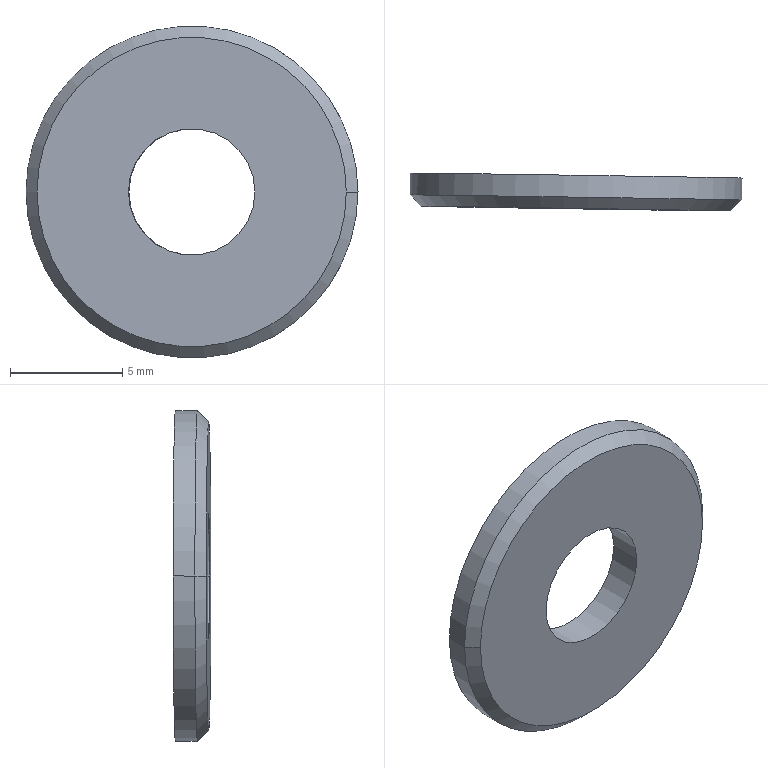Part | SolidWorks | features BaseBody 1 | 1 solid | 8 faces | box 14.798 x 1.69 x 14.785 mm | volume 210.71 mm3 | cylinder 4 | cone 2 | plane 2 | commonest cylinder face diameters 5.64 x2 14.785 x2
STEP:
#1=CARTESIAN_POINT('',(607.747,-33.383,255.544));
#2=VERTEX_POINT('',#1);
#3=CARTESIAN_POINT('',(602.108,-33.298,255.544));
#4=VERTEX_POINT('',#3);
#5=CARTESIAN_POINT('',(604.928,-33.341,255.544));
#6=DIRECTION('',(0.01505,0.9999,0.000000003));
#7=DIRECTION('',(-0.9999,0.01505,0.));
#8=AXIS2_PLACEMENT_3D('',#5,#6,#7);
#9=CIRCLE('',#8,2.82);
#10=EDGE_CURVE('',#2,#4,#9,.T.);
#11=ORIENTED_EDGE('',*,*,#10,.F.);
#12=CARTESIAN_POINT('',(607.77,-31.909,255.544));
#13=VERTEX_POINT('',#12);
#14=CARTESIAN_POINT('',(607.77,-31.909,255.544));
#15=DIRECTION('',(0.01505,0.9999,0.000000003));
#16=VECTOR('',#15,1000.);
#17=LINE('',#14,#16);
#18=EDGE_CURVE('',#2,#13,#17,.T.);
#19=ORIENTED_EDGE('',*,*,#18,.T.);
#20=CARTESIAN_POINT('',(602.13,-31.824,255.544));
#21=VERTEX_POINT('',#20);
#22=CARTESIAN_POINT('',(604.95,-31.866,255.544));
#23=DIRECTION('',(0.01505,0.9999,0.000000003));
#24=DIRECTION('',(-0.9999,0.01505,0.));
#25=AXIS2_PLACEMENT_3D('',#22,#23,#24);
#26=CIRCLE('',#25,2.82);
#27=EDGE_CURVE('',#13,#21,#26,.T.);
#28=ORIENTED_EDGE('',*,*,#27,.T.);
#29=CARTESIAN_POINT('',(602.13,-31.824,255.544));
#30=DIRECTION('',(0.01505,0.9999,0.000000003));
#31=VECTOR('',#30,1000.);
#32=LINE('',#29,#31);
#33=EDGE_CURVE('',#4,#21,#32,.T.);
#34=ORIENTED_EDGE('',*,*,#33,.F.);
#35=EDGE_LOOP('',(#11,#19,#28,#34));
#36=FACE_OUTER_BOUND('',#35,.T.);
#37=CARTESIAN_POINT('',(604.95,-31.866,255.544));
#38=DIRECTION('',(0.01505,0.9999,0.000000003));
#39=DIRECTION('',(-0.9999,0.01505,0.));
#40=AXIS2_PLACEMENT_3D('',#37,#38,#39);
#41=CYLINDRICAL_SURFACE('',#40,2.82);
#42=ADVANCED_FACE('',(#36),#41,.F.);
#43=CARTESIAN_POINT('',(597.544,-32.73,255.544));
#44=VERTEX_POINT('',#43);
#45=CARTESIAN_POINT('',(612.327,-32.952,255.544));
#46=VERTEX_POINT('',#45);
#47=CARTESIAN_POINT('',(604.935,-32.841,255.544));
#48=DIRECTION('',(0.01505,0.9999,0.000000003));
#49=DIRECTION('',(-0.9999,0.01505,0.));
#50=AXIS2_PLACEMENT_3D('',#47,#48,#49);
#51=CIRCLE('',#50,7.393);
#52=EDGE_CURVE('',#44,#46,#51,.T.);
#53=ORIENTED_EDGE('',*,*,#52,.T.);
#54=CARTESIAN_POINT('',(612.342,-31.977,255.544));
#55=VERTEX_POINT('',#54);
#56=CARTESIAN_POINT('',(612.342,-31.977,255.544));
#57=DIRECTION('',(0.01505,0.9999,0.000000003));
#58=VECTOR('',#57,1000.);
#59=LINE('',#56,#58);
#60=EDGE_CURVE('',#46,#55,#59,.T.);
#61=ORIENTED_EDGE('',*,*,#60,.T.);
#62=CARTESIAN_POINT('',(597.558,-31.755,255.544));
#63=VERTEX_POINT('',#62);
#64=CARTESIAN_POINT('',(604.95,-31.866,255.544));
#65=DIRECTION('',(-0.01505,-0.9999,-0.000000003));
#66=DIRECTION('',(-0.9999,0.01505,0.));
#67=AXIS2_PLACEMENT_3D('',#64,#65,#66);
#68=CIRCLE('',#67,7.393);
#69=EDGE_CURVE('',#55,#63,#68,.T.);
#70=ORIENTED_EDGE('',*,*,#69,.T.);
#71=CARTESIAN_POINT('',(597.558,-31.755,255.544));
#72=DIRECTION('',(0.01505,0.9999,0.000000003));
#73=VECTOR('',#72,1000.);
#74=LINE('',#71,#73);
#75=EDGE_CURVE('',#44,#63,#74,.T.);
#76=ORIENTED_EDGE('',*,*,#75,.F.);
#77=EDGE_LOOP('',(#53,#61,#70,#76));
#78=FACE_OUTER_BOUND('',#77,.T.);
#79=CARTESIAN_POINT('',(604.95,-31.866,255.544));
#80=DIRECTION('',(0.01505,0.9999,0.000000003));
#81=DIRECTION('',(-0.9999,0.01505,0.));
#82=AXIS2_PLACEMENT_3D('',#79,#80,#81);
#83=CYLINDRICAL_SURFACE('',#82,7.393);
#84=ADVANCED_FACE('',(#78),#83,.T.);
#85=CARTESIAN_POINT('',(611.82,-33.445,255.544));
#86=VERTEX_POINT('',#85);
#87=CARTESIAN_POINT('',(598.036,-33.237,255.544));
#88=VERTEX_POINT('',#87);
#89=CARTESIAN_POINT('',(604.928,-33.341,255.544));
#90=DIRECTION('',(-0.01505,-0.9999,-0.000000003));
#91=DIRECTION('',(-0.9999,0.01505,0.));
#92=AXIS2_PLACEMENT_3D('',#89,#90,#91);
#93=CIRCLE('',#92,6.892);
#94=EDGE_CURVE('',#86,#88,#93,.T.);
#95=ORIENTED_EDGE('',*,*,#94,.F.);
#96=CARTESIAN_POINT('',(612.327,-32.952,255.544));
#97=DIRECTION('',(0.7177,0.6964,0.000000002));
#98=VECTOR('',#97,1000.);
#99=LINE('',#96,#98);
#100=EDGE_CURVE('',#86,#46,#99,.T.);
#101=ORIENTED_EDGE('',*,*,#100,.T.);
#102=ORIENTED_EDGE('',*,*,#52,.F.);
#103=CARTESIAN_POINT('',(597.544,-32.73,255.544));
#104=DIRECTION('',(-0.6964,0.7177,0.000000002));
#105=VECTOR('',#104,1000.);
#106=LINE('',#103,#105);
#107=EDGE_CURVE('',#88,#44,#106,.T.);
#108=ORIENTED_EDGE('',*,*,#107,.F.);
#109=EDGE_LOOP('',(#95,#101,#102,#108));
#110=FACE_OUTER_BOUND('',#109,.T.);
#111=CARTESIAN_POINT('',(604.935,-32.841,255.544));
#112=DIRECTION('',(0.01505,0.9999,0.000000003));
#113=DIRECTION('',(-0.9999,0.01505,0.));
#114=AXIS2_PLACEMENT_3D('',#111,#112,#113);
#115=CONICAL_SURFACE('',#114,7.392,0.7854);
#116=ADVANCED_FACE('',(#110),#115,.T.);
#117=CARTESIAN_POINT('',(604.95,-31.866,255.544));
#118=DIRECTION('',(0.01505,0.9999,0.000000003));
#119=DIRECTION('',(-0.9999,0.01505,0.));
#120=AXIS2_PLACEMENT_3D('',#117,#118,#119);
#121=CIRCLE('',#120,2.82);
#122=EDGE_CURVE('',#21,#13,#121,.T.);
#123=ORIENTED_EDGE('',*,*,#122,.F.);
#124=ORIENTED_EDGE('',*,*,#27,.F.);
#125=EDGE_LOOP('',(#123,#124));
#126=FACE_BOUND('',#125,.T.);
#127=CARTESIAN_POINT('',(604.95,-31.866,255.544));
#128=DIRECTION('',(-0.01505,-0.9999,-0.000000003));
#129=DIRECTION('',(-0.9999,0.01505,0.));
#130=AXIS2_PLACEMENT_3D('',#127,#128,#129);
#131=CIRCLE('',#130,7.393);
#132=EDGE_CURVE('',#63,#55,#131,.T.);
#133=ORIENTED_EDGE('',*,*,#132,.F.);
#134=ORIENTED_EDGE('',*,*,#69,.F.);
#135=EDGE_LOOP('',(#133,#134));
#136=FACE_OUTER_BOUND('',#135,.T.);
#137=CARTESIAN_POINT('',(604.393,-31.858,255.532));
#138=DIRECTION('',(-0.01505,-0.9999,-0.000000003));
#139=DIRECTION('',(0.9999,-0.01505,0.));
#140=AXIS2_PLACEMENT_3D('',#137,#138,#139);
#141=PLANE('',#140);
#142=ADVANCED_FACE('',(#126,#136),#141,.F.);
#143=ORIENTED_EDGE('',*,*,#18,.F.);
#144=CARTESIAN_POINT('',(604.928,-33.341,255.544));
#145=DIRECTION('',(0.01505,0.9999,0.000000003));
#146=DIRECTION('',(-0.9999,0.01505,0.));
#147=AXIS2_PLACEMENT_3D('',#144,#145,#146);
#148=CIRCLE('',#147,2.82);
#149=EDGE_CURVE('',#4,#2,#148,.T.);
#150=ORIENTED_EDGE('',*,*,#149,.F.);
#151=ORIENTED_EDGE('',*,*,#33,.T.);
#152=ORIENTED_EDGE('',*,*,#122,.T.);
#153=EDGE_LOOP('',(#143,#150,#151,#152));
#154=FACE_OUTER_BOUND('',#153,.T.);
#155=CARTESIAN_POINT('',(604.95,-31.866,255.544));
#156=DIRECTION('',(0.01505,0.9999,0.000000003));
#157=DIRECTION('',(-0.9999,0.01505,0.));
#158=AXIS2_PLACEMENT_3D('',#155,#156,#157);
#159=CYLINDRICAL_SURFACE('',#158,2.82);
#160=ADVANCED_FACE('',(#154),#159,.F.);
#161=ORIENTED_EDGE('',*,*,#60,.F.);
#162=CARTESIAN_POINT('',(604.935,-32.841,255.544));
#163=DIRECTION('',(0.01505,0.9999,0.000000003));
#164=DIRECTION('',(-0.9999,0.01505,0.));
#165=AXIS2_PLACEMENT_3D('',#162,#163,#164);
#166=CIRCLE('',#165,7.393);
#167=EDGE_CURVE('',#46,#44,#166,.T.);
#168=ORIENTED_EDGE('',*,*,#167,.T.);
#169=ORIENTED_EDGE('',*,*,#75,.T.);
#170=ORIENTED_EDGE('',*,*,#132,.T.);
#171=EDGE_LOOP('',(#161,#168,#169,#170));
#172=FACE_OUTER_BOUND('',#171,.T.);
#173=CARTESIAN_POINT('',(604.95,-31.866,255.544));
#174=DIRECTION('',(0.01505,0.9999,0.000000003));
#175=DIRECTION('',(-0.9999,0.01505,0.));
#176=AXIS2_PLACEMENT_3D('',#173,#174,#175);
#177=CYLINDRICAL_SURFACE('',#176,7.393);
#178=ADVANCED_FACE('',(#172),#177,.T.);
#179=CARTESIAN_POINT('',(604.928,-33.341,255.544));
#180=DIRECTION('',(-0.01505,-0.9999,-0.000000003));
#181=DIRECTION('',(-0.9999,0.01505,0.));
#182=AXIS2_PLACEMENT_3D('',#179,#180,#181);
#183=CIRCLE('',#182,6.892);
#184=EDGE_CURVE('',#88,#86,#183,.T.);
#185=ORIENTED_EDGE('',*,*,#184,.T.);
#186=ORIENTED_EDGE('',*,*,#94,.T.);
#187=EDGE_LOOP('',(#185,#186));
#188=FACE_OUTER_BOUND('',#187,.T.);
#189=ORIENTED_EDGE('',*,*,#149,.T.);
#190=ORIENTED_EDGE('',*,*,#10,.T.);
#191=EDGE_LOOP('',(#189,#190));
#192=FACE_BOUND('',#191,.T.);
#193=CARTESIAN_POINT('',(604.371,-33.333,255.532));
#194=DIRECTION('',(-0.01505,-0.9999,-0.000000003));
#195=DIRECTION('',(0.9999,-0.01505,0.));
#196=AXIS2_PLACEMENT_3D('',#193,#194,#195);
#197=PLANE('',#196);
#198=ADVANCED_FACE('',(#188,#192),#197,.T.);
#199=ORIENTED_EDGE('',*,*,#100,.F.);
#200=ORIENTED_EDGE('',*,*,#184,.F.);
#201=ORIENTED_EDGE('',*,*,#107,.T.);
#202=ORIENTED_EDGE('',*,*,#167,.F.);
#203=EDGE_LOOP('',(#199,#200,#201,#202));
#204=FACE_OUTER_BOUND('',#203,.T.);
#205=CARTESIAN_POINT('',(604.935,-32.841,255.544));
#206=DIRECTION('',(0.01505,0.9999,0.000000003));
#207=DIRECTION('',(-0.9999,0.01505,0.));
#208=AXIS2_PLACEMENT_3D('',#205,#206,#207);
#209=CONICAL_SURFACE('',#208,7.392,0.7854);
#210=ADVANCED_FACE('',(#204),#209,.T.);
#211=CLOSED_SHELL('',(#42,#84,#116,#142,#160,#178,#198,#210));
#212=MANIFOLD_SOLID_BREP('',#211);
#213=CARTESIAN_POINT('',(0.,0.,0.));
#214=DIRECTION('',(0.,0.,1.));
#215=DIRECTION('',(1.,0.,0.));
#216=AXIS2_PLACEMENT_3D('',#213,#214,#215);
#217=(LENGTH_UNIT()NAMED_UNIT(*)SI_UNIT(.MILLI.,.METRE.));
#218=UNCERTAINTY_MEASURE_WITH_UNIT(LENGTH_MEASURE(0.00001),#217,'','');
#219=(NAMED_UNIT(*)PLANE_ANGLE_UNIT()SI_UNIT($,.RADIAN.));
#220=(NAMED_UNIT(*)SI_UNIT($,.STERADIAN.)SOLID_ANGLE_UNIT());
#221=(GEOMETRIC_REPRESENTATION_CONTEXT(3)GLOBAL_UNCERTAINTY_ASSIGNED_CONTEXT((#218))GLOBAL_UNIT_ASSIGNED_CONTEXT((#217,#219,#220))REPRESENTATION_CONTEXT('',''));
#222=ADVANCED_BREP_SHAPE_REPRESENTATION('',(#212,#216),#221);